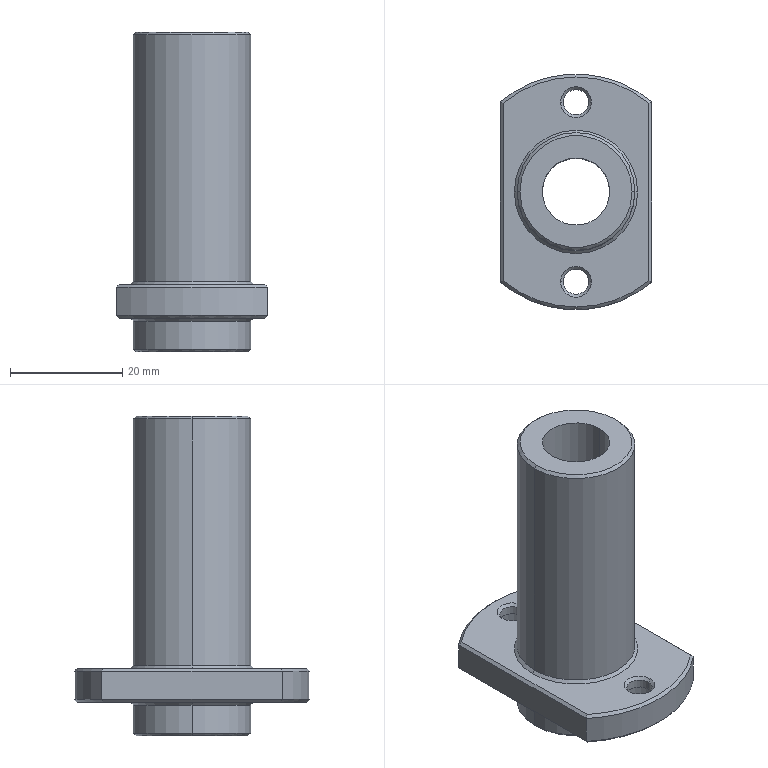Part | SolidWorks | features ICE 4, Chamfer 2, Extrusion 1, HoleWzd 1 | 1 solid | 48 faces | box 27 x 42 x 57 mm | volume 17013 mm3 | cone 20 | cylinder 16 | plane 12 | commonest cylinder face diameters 4.5 x4 8 x4 21 x4 12 x2 42 x2
STEP:
#1=CARTESIAN_POINT('',(4.,16.,6.5));
#2=VERTEX_POINT('',#1);
#3=CARTESIAN_POINT('',(-4.,16.,6.5));
#4=VERTEX_POINT('',#3);
#5=CARTESIAN_POINT('',(0.,16.,6.5));
#6=DIRECTION('',(0.,0.,-1.));
#7=DIRECTION('',(1.,0.,0.));
#8=AXIS2_PLACEMENT_3D('',#5,#6,#7);
#9=CIRCLE('',#8,4.);
#10=EDGE_CURVE('',#2,#4,#9,.T.);
#11=ORIENTED_EDGE('',*,*,#10,.F.);
#12=CARTESIAN_POINT('',(4.5,16.,6.));
#13=VERTEX_POINT('',#12);
#14=CARTESIAN_POINT('',(4.,16.,6.5));
#15=DIRECTION('',(0.7071,0.,-0.7071));
#16=VECTOR('',#15,1000.);
#17=LINE('',#14,#16);
#18=EDGE_CURVE('',#2,#13,#17,.T.);
#19=ORIENTED_EDGE('',*,*,#18,.T.);
#20=CARTESIAN_POINT('',(-4.5,16.,6.));
#21=VERTEX_POINT('',#20);
#22=CARTESIAN_POINT('',(0.,16.,6.));
#23=DIRECTION('',(0.,0.,1.));
#24=DIRECTION('',(1.,0.,0.));
#25=AXIS2_PLACEMENT_3D('',#22,#23,#24);
#26=CIRCLE('',#25,4.5);
#27=EDGE_CURVE('',#21,#13,#26,.T.);
#28=ORIENTED_EDGE('',*,*,#27,.F.);
#29=CARTESIAN_POINT('',(-4.,16.,6.5));
#30=DIRECTION('',(-0.7071,0.,-0.7071));
#31=VECTOR('',#30,1000.);
#32=LINE('',#29,#31);
#33=EDGE_CURVE('',#4,#21,#32,.T.);
#34=ORIENTED_EDGE('',*,*,#33,.F.);
#35=EDGE_LOOP('',(#11,#19,#28,#34));
#36=FACE_OUTER_BOUND('',#35,.T.);
#37=CARTESIAN_POINT('',(0.,16.,6.5));
#38=DIRECTION('',(0.,0.,-1.));
#39=DIRECTION('',(-1.,0.,0.));
#40=AXIS2_PLACEMENT_3D('',#37,#38,#39);
#41=CONICAL_SURFACE('',#40,4.,0.7854);
#42=ADVANCED_FACE('',(#36),#41,.F.);
#43=CARTESIAN_POINT('',(4.,-16.,6.5));
#44=VERTEX_POINT('',#43);
#45=CARTESIAN_POINT('',(-4.,-16.,6.5));
#46=VERTEX_POINT('',#45);
#47=CARTESIAN_POINT('',(0.,-16.,6.5));
#48=DIRECTION('',(0.,0.,-1.));
#49=DIRECTION('',(1.,0.,0.));
#50=AXIS2_PLACEMENT_3D('',#47,#48,#49);
#51=CIRCLE('',#50,4.);
#52=EDGE_CURVE('',#44,#46,#51,.T.);
#53=ORIENTED_EDGE('',*,*,#52,.F.);
#54=CARTESIAN_POINT('',(4.5,-16.,6.));
#55=VERTEX_POINT('',#54);
#56=CARTESIAN_POINT('',(4.,-16.,6.5));
#57=DIRECTION('',(0.7071,0.,-0.7071));
#58=VECTOR('',#57,1000.);
#59=LINE('',#56,#58);
#60=EDGE_CURVE('',#44,#55,#59,.T.);
#61=ORIENTED_EDGE('',*,*,#60,.T.);
#62=CARTESIAN_POINT('',(0.,-20.5,6.));
#63=VERTEX_POINT('',#62);
#64=CARTESIAN_POINT('',(0.,-16.,6.));
#65=DIRECTION('',(0.,0.,1.));
#66=DIRECTION('',(1.,0.,0.));
#67=AXIS2_PLACEMENT_3D('',#64,#65,#66);
#68=CIRCLE('',#67,4.5);
#69=EDGE_CURVE('',#63,#55,#68,.T.);
#70=ORIENTED_EDGE('',*,*,#69,.F.);
#71=CARTESIAN_POINT('',(-4.5,-16.,6.));
#72=VERTEX_POINT('',#71);
#73=CARTESIAN_POINT('',(0.,-16.,6.));
#74=DIRECTION('',(0.,0.,1.));
#75=DIRECTION('',(1.,0.,0.));
#76=AXIS2_PLACEMENT_3D('',#73,#74,#75);
#77=CIRCLE('',#76,4.5);
#78=EDGE_CURVE('',#72,#63,#77,.T.);
#79=ORIENTED_EDGE('',*,*,#78,.F.);
#80=CARTESIAN_POINT('',(-4.,-16.,6.5));
#81=DIRECTION('',(-0.7071,0.,-0.7071));
#82=VECTOR('',#81,1000.);
#83=LINE('',#80,#82);
#84=EDGE_CURVE('',#46,#72,#83,.T.);
#85=ORIENTED_EDGE('',*,*,#84,.F.);
#86=EDGE_LOOP('',(#53,#61,#70,#79,#85));
#87=FACE_OUTER_BOUND('',#86,.T.);
#88=CARTESIAN_POINT('',(0.,-16.,6.5));
#89=DIRECTION('',(0.,0.,-1.));
#90=DIRECTION('',(-1.,0.,0.));
#91=AXIS2_PLACEMENT_3D('',#88,#89,#90);
#92=CONICAL_SURFACE('',#91,4.,0.7854);
#93=ADVANCED_FACE('',(#87),#92,.F.);
#94=CARTESIAN_POINT('',(-10.5,0.,5.5));
#95=VERTEX_POINT('',#94);
#96=CARTESIAN_POINT('',(10.5,0.,5.5));
#97=VERTEX_POINT('',#96);
#98=CARTESIAN_POINT('',(0.,0.,5.5));
#99=DIRECTION('',(0.,0.,-1.));
#100=DIRECTION('',(1.,0.,0.));
#101=AXIS2_PLACEMENT_3D('',#98,#99,#100);
#102=CIRCLE('',#101,10.5);
#103=EDGE_CURVE('',#95,#97,#102,.T.);
#104=ORIENTED_EDGE('',*,*,#103,.F.);
#105=CARTESIAN_POINT('',(-11.,0.,6.));
#106=VERTEX_POINT('',#105);
#107=CARTESIAN_POINT('',(-11.,0.,6.));
#108=DIRECTION('',(-0.7071,0.,0.7071));
#109=VECTOR('',#108,1000.);
#110=LINE('',#107,#109);
#111=EDGE_CURVE('',#95,#106,#110,.T.);
#112=ORIENTED_EDGE('',*,*,#111,.T.);
#113=CARTESIAN_POINT('',(11.,0.,6.));
#114=VERTEX_POINT('',#113);
#115=CARTESIAN_POINT('',(0.,0.,6.));
#116=DIRECTION('',(0.,0.,1.));
#117=DIRECTION('',(1.,0.,0.));
#118=AXIS2_PLACEMENT_3D('',#115,#116,#117);
#119=CIRCLE('',#118,11.);
#120=EDGE_CURVE('',#114,#106,#119,.T.);
#121=ORIENTED_EDGE('',*,*,#120,.F.);
#122=CARTESIAN_POINT('',(11.,0.,6.));
#123=DIRECTION('',(0.7071,0.,0.7071));
#124=VECTOR('',#123,1000.);
#125=LINE('',#122,#124);
#126=EDGE_CURVE('',#97,#114,#125,.T.);
#127=ORIENTED_EDGE('',*,*,#126,.F.);
#128=EDGE_LOOP('',(#104,#112,#121,#127));
#129=FACE_OUTER_BOUND('',#128,.T.);
#130=CARTESIAN_POINT('',(0.,0.,6.));
#131=DIRECTION('',(0.,0.,1.));
#132=DIRECTION('',(1.,0.,0.));
#133=AXIS2_PLACEMENT_3D('',#130,#131,#132);
#134=CONICAL_SURFACE('',#133,11.,0.7854);
#135=ADVANCED_FACE('',(#129),#134,.T.);
#136=CARTESIAN_POINT('',(-2.25,16.,11.5));
#137=VERTEX_POINT('',#136);
#138=CARTESIAN_POINT('',(2.25,16.,11.5));
#139=VERTEX_POINT('',#138);
#140=CARTESIAN_POINT('',(0.,16.,11.5));
#141=DIRECTION('',(0.,0.,1.));
#142=DIRECTION('',(1.,0.,0.));
#143=AXIS2_PLACEMENT_3D('',#140,#141,#142);
#144=CIRCLE('',#143,2.25);
#145=EDGE_CURVE('',#137,#139,#144,.T.);
#146=ORIENTED_EDGE('',*,*,#145,.F.);
#147=CARTESIAN_POINT('',(-2.75,16.,12.));
#148=VERTEX_POINT('',#147);
#149=CARTESIAN_POINT('',(-2.25,16.,11.5));
#150=DIRECTION('',(-0.7071,0.,0.7071));
#151=VECTOR('',#150,1000.);
#152=LINE('',#149,#151);
#153=EDGE_CURVE('',#137,#148,#152,.T.);
#154=ORIENTED_EDGE('',*,*,#153,.T.);
#155=CARTESIAN_POINT('',(2.75,16.,12.));
#156=VERTEX_POINT('',#155);
#157=CARTESIAN_POINT('',(0.,16.,12.));
#158=DIRECTION('',(0.,0.,-1.));
#159=DIRECTION('',(1.,0.,0.));
#160=AXIS2_PLACEMENT_3D('',#157,#158,#159);
#161=CIRCLE('',#160,2.75);
#162=EDGE_CURVE('',#156,#148,#161,.T.);
#163=ORIENTED_EDGE('',*,*,#162,.F.);
#164=CARTESIAN_POINT('',(2.25,16.,11.5));
#165=DIRECTION('',(0.7071,0.,0.7071));
#166=VECTOR('',#165,1000.);
#167=LINE('',#164,#166);
#168=EDGE_CURVE('',#139,#156,#167,.T.);
#169=ORIENTED_EDGE('',*,*,#168,.F.);
#170=EDGE_LOOP('',(#146,#154,#163,#169));
#171=FACE_OUTER_BOUND('',#170,.T.);
#172=CARTESIAN_POINT('',(0.,16.,11.5));
#173=DIRECTION('',(0.,0.,1.));
#174=DIRECTION('',(1.,0.,0.));
#175=AXIS2_PLACEMENT_3D('',#172,#173,#174);
#176=CONICAL_SURFACE('',#175,2.25,0.7854);
#177=ADVANCED_FACE('',(#171),#176,.F.);
#178=CARTESIAN_POINT('',(-2.25,-16.,11.5));
#179=VERTEX_POINT('',#178);
#180=CARTESIAN_POINT('',(2.25,-16.,11.5));
#181=VERTEX_POINT('',#180);
#182=CARTESIAN_POINT('',(0.,-16.,11.5));
#183=DIRECTION('',(0.,0.,1.));
#184=DIRECTION('',(1.,0.,0.));
#185=AXIS2_PLACEMENT_3D('',#182,#183,#184);
#186=CIRCLE('',#185,2.25);
#187=EDGE_CURVE('',#179,#181,#186,.T.);
#188=ORIENTED_EDGE('',*,*,#187,.F.);
#189=CARTESIAN_POINT('',(-2.75,-16.,12.));
#190=VERTEX_POINT('',#189);
#191=CARTESIAN_POINT('',(-2.25,-16.,11.5));
#192=DIRECTION('',(-0.7071,0.,0.7071));
#193=VECTOR('',#192,1000.);
#194=LINE('',#191,#193);
#195=EDGE_CURVE('',#179,#190,#194,.T.);
#196=ORIENTED_EDGE('',*,*,#195,.T.);
#197=CARTESIAN_POINT('',(2.75,-16.,12.));
#198=VERTEX_POINT('',#197);
#199=CARTESIAN_POINT('',(0.,-16.,12.));
#200=DIRECTION('',(0.,0.,-1.));
#201=DIRECTION('',(1.,0.,0.));
#202=AXIS2_PLACEMENT_3D('',#199,#200,#201);
#203=CIRCLE('',#202,2.75);
#204=EDGE_CURVE('',#198,#190,#203,.T.);
#205=ORIENTED_EDGE('',*,*,#204,.F.);
#206=CARTESIAN_POINT('',(2.25,-16.,11.5));
#207=DIRECTION('',(0.7071,0.,0.7071));
#208=VECTOR('',#207,1000.);
#209=LINE('',#206,#208);
#210=EDGE_CURVE('',#181,#198,#209,.T.);
#211=ORIENTED_EDGE('',*,*,#210,.F.);
#212=EDGE_LOOP('',(#188,#196,#205,#211));
#213=FACE_OUTER_BOUND('',#212,.T.);
#214=CARTESIAN_POINT('',(0.,-16.,11.5));
#215=DIRECTION('',(0.,0.,1.));
#216=DIRECTION('',(1.,0.,0.));
#217=AXIS2_PLACEMENT_3D('',#214,#215,#216);
#218=CONICAL_SURFACE('',#217,2.25,0.7854);
#219=ADVANCED_FACE('',(#213),#218,.F.);
#220=CARTESIAN_POINT('',(10.5,0.,12.5));
#221=VERTEX_POINT('',#220);
#222=CARTESIAN_POINT('',(-10.5,0.,12.5));
#223=VERTEX_POINT('',#222);
#224=CARTESIAN_POINT('',(0.,0.,12.5));
#225=DIRECTION('',(0.,0.,1.));
#226=DIRECTION('',(1.,0.,0.));
#227=AXIS2_PLACEMENT_3D('',#224,#225,#226);
#228=CIRCLE('',#227,10.5);
#229=EDGE_CURVE('',#221,#223,#228,.T.);
#230=ORIENTED_EDGE('',*,*,#229,.F.);
#231=CARTESIAN_POINT('',(11.,0.,12.));
#232=VERTEX_POINT('',#231);
#233=CARTESIAN_POINT('',(10.5,0.,12.5));
#234=DIRECTION('',(0.7071,0.,-0.7071));
#235=VECTOR('',#234,1000.);
#236=LINE('',#233,#235);
#237=EDGE_CURVE('',#221,#232,#236,.T.);
#238=ORIENTED_EDGE('',*,*,#237,.T.);
#239=CARTESIAN_POINT('',(-11.,0.,12.));
#240=VERTEX_POINT('',#239);
#241=CARTESIAN_POINT('',(0.,0.,12.));
#242=DIRECTION('',(0.,0.,-1.));
#243=DIRECTION('',(1.,0.,0.));
#244=AXIS2_PLACEMENT_3D('',#241,#242,#243);
#245=CIRCLE('',#244,11.);
#246=EDGE_CURVE('',#240,#232,#245,.T.);
#247=ORIENTED_EDGE('',*,*,#246,.F.);
#248=CARTESIAN_POINT('',(-10.5,0.,12.5));
#249=DIRECTION('',(-0.7071,0.,-0.7071));
#250=VECTOR('',#249,1000.);
#251=LINE('',#248,#250);
#252=EDGE_CURVE('',#223,#240,#251,.T.);
#253=ORIENTED_EDGE('',*,*,#252,.F.);
#254=EDGE_LOOP('',(#230,#238,#247,#253));
#255=FACE_OUTER_BOUND('',#254,.T.);
#256=CARTESIAN_POINT('',(0.,0.,12.5));
#257=DIRECTION('',(0.,0.,-1.));
#258=DIRECTION('',(-1.,0.,0.));
#259=AXIS2_PLACEMENT_3D('',#256,#257,#258);
#260=CONICAL_SURFACE('',#259,10.5,0.7854);
#261=ADVANCED_FACE('',(#255),#260,.T.);
#262=CARTESIAN_POINT('',(10.,0.,57.));
#263=VERTEX_POINT('',#262);
#264=CARTESIAN_POINT('',(-10.,0.,57.));
#265=VERTEX_POINT('',#264);
#266=CARTESIAN_POINT('',(0.,0.,57.));
#267=DIRECTION('',(0.,0.,1.));
#268=DIRECTION('',(1.,0.,0.));
#269=AXIS2_PLACEMENT_3D('',#266,#267,#268);
#270=CIRCLE('',#269,10.);
#271=EDGE_CURVE('',#263,#265,#270,.T.);
#272=ORIENTED_EDGE('',*,*,#271,.F.);
#273=CARTESIAN_POINT('',(10.5,0.,56.5));
#274=VERTEX_POINT('',#273);
#275=CARTESIAN_POINT('',(10.,0.,57.));
#276=DIRECTION('',(0.7071,0.,-0.7071));
#277=VECTOR('',#276,1000.);
#278=LINE('',#275,#277);
#279=EDGE_CURVE('',#263,#274,#278,.T.);
#280=ORIENTED_EDGE('',*,*,#279,.T.);
#281=CARTESIAN_POINT('',(-10.5,0.,56.5));
#282=VERTEX_POINT('',#281);
#283=CARTESIAN_POINT('',(0.,0.,56.5));
#284=DIRECTION('',(0.,0.,-1.));
#285=DIRECTION('',(1.,0.,0.));
#286=AXIS2_PLACEMENT_3D('',#283,#284,#285);
#287=CIRCLE('',#286,10.5);
#288=EDGE_CURVE('',#282,#274,#287,.T.);
#289=ORIENTED_EDGE('',*,*,#288,.F.);
#290=CARTESIAN_POINT('',(-10.,0.,57.));
#291=DIRECTION('',(-0.7071,0.,-0.7071));
#292=VECTOR('',#291,1000.);
#293=LINE('',#290,#292);
#294=EDGE_CURVE('',#265,#282,#293,.T.);
#295=ORIENTED_EDGE('',*,*,#294,.F.);
#296=EDGE_LOOP('',(#272,#280,#289,#295));
#297=FACE_OUTER_BOUND('',#296,.T.);
#298=CARTESIAN_POINT('',(0.,0.,57.));
#299=DIRECTION('',(0.,0.,-1.));
#300=DIRECTION('',(-1.,0.,0.));
#301=AXIS2_PLACEMENT_3D('',#298,#299,#300);
#302=CONICAL_SURFACE('',#301,10.,0.7854);
#303=ADVANCED_FACE('',(#297),#302,.T.);
#304=CARTESIAN_POINT('',(-10.,0.,0.));
#305=VERTEX_POINT('',#304);
#306=CARTESIAN_POINT('',(10.,0.,0.));
#307=VERTEX_POINT('',#306);
#308=CARTESIAN_POINT('',(0.,0.,0.));
#309=DIRECTION('',(0.,0.,-1.));
#310=DIRECTION('',(1.,0.,0.));
#311=AXIS2_PLACEMENT_3D('',#308,#309,#310);
#312=CIRCLE('',#311,10.);
#313=EDGE_CURVE('',#305,#307,#312,.T.);
#314=ORIENTED_EDGE('',*,*,#313,.F.);
#315=CARTESIAN_POINT('',(-10.5,0.,0.5));
#316=VERTEX_POINT('',#315);
#317=CARTESIAN_POINT('',(-10.5,0.,0.5));
#318=DIRECTION('',(-0.7071,0.,0.7071));
#319=VECTOR('',#318,1000.);
#320=LINE('',#317,#319);
#321=EDGE_CURVE('',#305,#316,#320,.T.);
#322=ORIENTED_EDGE('',*,*,#321,.T.);
#323=CARTESIAN_POINT('',(10.5,0.,0.5));
#324=VERTEX_POINT('',#323);
#325=CARTESIAN_POINT('',(0.,0.,0.5));
#326=DIRECTION('',(0.,0.,1.));
#327=DIRECTION('',(1.,0.,0.));
#328=AXIS2_PLACEMENT_3D('',#325,#326,#327);
#329=CIRCLE('',#328,10.5);
#330=EDGE_CURVE('',#324,#316,#329,.T.);
#331=ORIENTED_EDGE('',*,*,#330,.F.);
#332=CARTESIAN_POINT('',(10.5,0.,0.5));
#333=DIRECTION('',(0.7071,0.,0.7071));
#334=VECTOR('',#333,1000.);
#335=LINE('',#332,#334);
#336=EDGE_CURVE('',#307,#324,#335,.T.);
#337=ORIENTED_EDGE('',*,*,#336,.F.);
#338=EDGE_LOOP('',(#314,#322,#331,#337));
#339=FACE_OUTER_BOUND('',#338,.T.);
#340=CARTESIAN_POINT('',(0.,0.,0.5));
#341=DIRECTION('',(0.,0.,1.));
#342=DIRECTION('',(1.,0.,0.));
#343=AXIS2_PLACEMENT_3D('',#340,#341,#342);
#344=CONICAL_SURFACE('',#343,10.5,0.7854);
#345=ADVANCED_FACE('',(#339),#344,.T.);
#346=CARTESIAN_POINT('',(4.,16.,10.));
#347=VERTEX_POINT('',#346);
#348=CARTESIAN_POINT('',(-4.,16.,10.));
#349=VERTEX_POINT('',#348);
#350=CARTESIAN_POINT('',(0.,16.,10.));
#351=DIRECTION('',(0.,0.,-1.));
#352=DIRECTION('',(-1.,0.,0.));
#353=AXIS2_PLACEMENT_3D('',#350,#351,#352);
#354=CIRCLE('',#353,4.);
#355=EDGE_CURVE('',#347,#349,#354,.T.);
#356=ORIENTED_EDGE('',*,*,#355,.F.);
#357=CARTESIAN_POINT('',(4.,16.,6.));
#358=DIRECTION('',(0.,0.,-1.));
#359=VECTOR('',#358,1000.);
#360=LINE('',#357,#359);
#361=EDGE_CURVE('',#347,#2,#360,.T.);
#362=ORIENTED_EDGE('',*,*,#361,.T.);
#363=ORIENTED_EDGE('',*,*,#10,.T.);
#364=CARTESIAN_POINT('',(-4.,16.,6.));
#365=DIRECTION('',(0.,0.,-1.));
#366=VECTOR('',#365,1000.);
#367=LINE('',#364,#366);
#368=EDGE_CURVE('',#349,#4,#367,.T.);
#369=ORIENTED_EDGE('',*,*,#368,.F.);
#370=EDGE_LOOP('',(#356,#362,#363,#369));
#371=FACE_OUTER_BOUND('',#370,.T.);
#372=CARTESIAN_POINT('',(0.,16.,6.));
#373=DIRECTION('',(0.,0.,-1.));
#374=DIRECTION('',(-1.,0.,0.));
#375=AXIS2_PLACEMENT_3D('',#372,#373,#374);
#376=CYLINDRICAL_SURFACE('',#375,4.);
#377=ADVANCED_FACE('',(#371),#376,.F.);
#378=ORIENTED_EDGE('',*,*,#145,.T.);
#379=CARTESIAN_POINT('',(2.25,16.,10.));
#380=VERTEX_POINT('',#379);
#381=CARTESIAN_POINT('',(2.25,16.,6.));
#382=DIRECTION('',(0.,0.,-1.));
#383=VECTOR('',#382,1000.);
#384=LINE('',#381,#383);
#385=EDGE_CURVE('',#139,#380,#384,.T.);
#386=ORIENTED_EDGE('',*,*,#385,.T.);
#387=CARTESIAN_POINT('',(-2.25,16.,10.));
#388=VERTEX_POINT('',#387);
#389=CARTESIAN_POINT('',(0.,16.,10.));
#390=DIRECTION('',(0.,0.,-1.));
#391=DIRECTION('',(-1.,0.,0.));
#392=AXIS2_PLACEMENT_3D('',#389,#390,#391);
#393=CIRCLE('',#392,2.25);
#394=EDGE_CURVE('',#380,#388,#393,.T.);
#395=ORIENTED_EDGE('',*,*,#394,.T.);
#396=CARTESIAN_POINT('',(-2.25,16.,6.));
#397=DIRECTION('',(0.,0.,-1.));
#398=VECTOR('',#397,1000.);
#399=LINE('',#396,#398);
#400=EDGE_CURVE('',#137,#388,#399,.T.);
#401=ORIENTED_EDGE('',*,*,#400,.F.);
#402=EDGE_LOOP('',(#378,#386,#395,#401));
#403=FACE_OUTER_BOUND('',#402,.T.);
#404=CARTESIAN_POINT('',(0.,16.,6.));
#405=DIRECTION('',(0.,0.,-1.));
#406=DIRECTION('',(-1.,0.,0.));
#407=AXIS2_PLACEMENT_3D('',#404,#405,#406);
#408=CYLINDRICAL_SURFACE('',#407,2.25);
#409=ADVANCED_FACE('',(#403),#408,.F.);
#410=CARTESIAN_POINT('',(4.,-16.,10.));
#411=VERTEX_POINT('',#410);
#412=CARTESIAN_POINT('',(-4.,-16.,10.));
#413=VERTEX_POINT('',#412);
#414=CARTESIAN_POINT('',(0.,-16.,10.));
#415=DIRECTION('',(0.,0.,-1.));
#416=DIRECTION('',(-1.,0.,0.));
#417=AXIS2_PLACEMENT_3D('',#414,#415,#416);
#418=CIRCLE('',#417,4.);
#419=EDGE_CURVE('',#411,#413,#418,.T.);
#420=ORIENTED_EDGE('',*,*,#419,.F.);
#421=CARTESIAN_POINT('',(4.,-16.,6.));
#422=DIRECTION('',(0.,0.,-1.));
#423=VECTOR('',#422,1000.);
#424=LINE('',#421,#423);
#425=EDGE_CURVE('',#411,#44,#424,.T.);
#426=ORIENTED_EDGE('',*,*,#425,.T.);
#427=ORIENTED_EDGE('',*,*,#52,.T.);
#428=CARTESIAN_POINT('',(-4.,-16.,6.));
#429=DIRECTION('',(0.,0.,-1.));
#430=VECTOR('',#429,1000.);
#431=LINE('',#428,#430);
#432=EDGE_CURVE('',#413,#46,#431,.T.);
#433=ORIENTED_EDGE('',*,*,#432,.F.);
#434=EDGE_LOOP('',(#420,#426,#427,#433));
#435=FACE_OUTER_BOUND('',#434,.T.);
#436=CARTESIAN_POINT('',(0.,-16.,6.));
#437=DIRECTION('',(0.,0.,-1.));
#438=DIRECTION('',(-1.,0.,0.));
#439=AXIS2_PLACEMENT_3D('',#436,#437,#438);
#440=CYLINDRICAL_SURFACE('',#439,4.);
#441=ADVANCED_FACE('',(#435),#440,.F.);
#442=ORIENTED_EDGE('',*,*,#187,.T.);
#443=CARTESIAN_POINT('',(2.25,-16.,10.));
#444=VERTEX_POINT('',#443);
#445=CARTESIAN_POINT('',(2.25,-16.,6.));
#446=DIRECTION('',(0.,0.,-1.));
#447=VECTOR('',#446,1000.);
#448=LINE('',#445,#447);
#449=EDGE_CURVE('',#181,#444,#448,.T.);
#450=ORIENTED_EDGE('',*,*,#449,.T.);
#451=CARTESIAN_POINT('',(-2.25,-16.,10.));
#452=VERTEX_POINT('',#451);
#453=CARTESIAN_POINT('',(0.,-16.,10.));
#454=DIRECTION('',(0.,0.,-1.));
#455=DIRECTION('',(-1.,0.,0.));
#456=AXIS2_PLACEMENT_3D('',#453,#454,#455);
#457=CIRCLE('',#456,2.25);
#458=EDGE_CURVE('',#444,#452,#457,.T.);
#459=ORIENTED_EDGE('',*,*,#458,.T.);
#460=CARTESIAN_POINT('',(-2.25,-16.,6.));
#461=DIRECTION('',(0.,0.,-1.));
#462=VECTOR('',#461,1000.);
#463=LINE('',#460,#462);
#464=EDGE_CURVE('',#179,#452,#463,.T.);
#465=ORIENTED_EDGE('',*,*,#464,.F.);
#466=EDGE_LOOP('',(#442,#450,#459,#465));
#467=FACE_OUTER_BOUND('',#466,.T.);
#468=CARTESIAN_POINT('',(0.,-16.,6.));
#469=DIRECTION('',(0.,0.,-1.));
#470=DIRECTION('',(-1.,0.,0.));
#471=AXIS2_PLACEMENT_3D('',#468,#469,#470);
#472=CYLINDRICAL_SURFACE('',#471,2.25);
#473=ADVANCED_FACE('',(#467),#472,.F.);
#474=CARTESIAN_POINT('',(-6.,0.,0.));
#475=VERTEX_POINT('',#474);
#476=CARTESIAN_POINT('',(6.,0.,0.));
#477=VERTEX_POINT('',#476);
#478=CARTESIAN_POINT('',(0.,0.,0.));
#479=DIRECTION('',(0.,0.,1.));
#480=DIRECTION('',(1.,0.,0.));
#481=AXIS2_PLACEMENT_3D('',#478,#479,#480);
#482=CIRCLE('',#481,6.);
#483=EDGE_CURVE('',#475,#477,#482,.T.);
#484=ORIENTED_EDGE('',*,*,#483,.F.);
#485=CARTESIAN_POINT('',(-6.,0.,57.));
#486=VERTEX_POINT('',#485);
#487=CARTESIAN_POINT('',(-6.,0.,0.));
#488=DIRECTION('',(0.,0.,1.));
#489=VECTOR('',#488,1000.);
#490=LINE('',#487,#489);
#491=EDGE_CURVE('',#475,#486,#490,.T.);
#492=ORIENTED_EDGE('',*,*,#491,.T.);
#493=CARTESIAN_POINT('',(6.,0.,57.));
#494=VERTEX_POINT('',#493);
#495=CARTESIAN_POINT('',(0.,0.,57.));
#496=DIRECTION('',(0.,0.,1.));
#497=DIRECTION('',(1.,0.,0.));
#498=AXIS2_PLACEMENT_3D('',#495,#496,#497);
#499=CIRCLE('',#498,6.);
#500=EDGE_CURVE('',#486,#494,#499,.T.);
#501=ORIENTED_EDGE('',*,*,#500,.T.);
#502=CARTESIAN_POINT('',(6.,0.,0.));
#503=DIRECTION('',(0.,0.,1.));
#504=VECTOR('',#503,1000.);
#505=LINE('',#502,#504);
#506=EDGE_CURVE('',#477,#494,#505,.T.);
#507=ORIENTED_EDGE('',*,*,#506,.F.);
#508=EDGE_LOOP('',(#484,#492,#501,#507));
#509=FACE_OUTER_BOUND('',#508,.T.);
#510=CARTESIAN_POINT('',(0.,0.,0.));
#511=DIRECTION('',(0.,0.,1.));
#512=DIRECTION('',(1.,0.,0.));
#513=AXIS2_PLACEMENT_3D('',#510,#511,#512);
#514=CYLINDRICAL_SURFACE('',#513,6.);
#515=ADVANCED_FACE('',(#509),#514,.F.);
#516=ORIENTED_EDGE('',*,*,#288,.T.);
#517=CARTESIAN_POINT('',(10.5,0.,57.));
#518=DIRECTION('',(0.,0.,-1.));
#519=VECTOR('',#518,1000.);
#520=LINE('',#517,#519);
#521=EDGE_CURVE('',#274,#221,#520,.T.);
#522=ORIENTED_EDGE('',*,*,#521,.T.);
#523=ORIENTED_EDGE('',*,*,#229,.T.);
#524=CARTESIAN_POINT('',(-10.5,0.,57.));
#525=DIRECTION('',(0.,0.,-1.));
#526=VECTOR('',#525,1000.);
#527=LINE('',#524,#526);
#528=EDGE_CURVE('',#282,#223,#527,.T.);
#529=ORIENTED_EDGE('',*,*,#528,.F.);
#530=EDGE_LOOP('',(#516,#522,#523,#529));
#531=FACE_OUTER_BOUND('',#530,.T.);
#532=CARTESIAN_POINT('',(0.,0.,57.));
#533=DIRECTION('',(0.,0.,-1.));
#534=DIRECTION('',(-1.,0.,0.));
#535=AXIS2_PLACEMENT_3D('',#532,#533,#534);
#536=CYLINDRICAL_SURFACE('',#535,10.5);
#537=ADVANCED_FACE('',(#531),#536,.T.);
#538=ORIENTED_EDGE('',*,*,#103,.T.);
#539=CARTESIAN_POINT('',(10.5,0.,6.));
#540=DIRECTION('',(0.,0.,-1.));
#541=VECTOR('',#540,1000.);
#542=LINE('',#539,#541);
#543=EDGE_CURVE('',#97,#324,#542,.T.);
#544=ORIENTED_EDGE('',*,*,#543,.T.);
#545=ORIENTED_EDGE('',*,*,#330,.T.);
#546=CARTESIAN_POINT('',(-10.5,0.,6.));
#547=DIRECTION('',(0.,0.,-1.));
#548=VECTOR('',#547,1000.);
#549=LINE('',#546,#548);
#550=EDGE_CURVE('',#95,#316,#549,.T.);
#551=ORIENTED_EDGE('',*,*,#550,.F.);
#552=EDGE_LOOP('',(#538,#544,#545,#551));
#553=FACE_OUTER_BOUND('',#552,.T.);
#554=CARTESIAN_POINT('',(0.,0.,6.));
#555=DIRECTION('',(0.,0.,-1.));
#556=DIRECTION('',(-1.,0.,0.));
#557=AXIS2_PLACEMENT_3D('',#554,#555,#556);
#558=CYLINDRICAL_SURFACE('',#557,10.5);
#559=ADVANCED_FACE('',(#553),#558,.T.);
#560=CARTESIAN_POINT('',(13.,15.851,12.));
#561=VERTEX_POINT('',#560);
#562=CARTESIAN_POINT('',(-13.,15.851,12.));
#563=VERTEX_POINT('',#562);
#564=CARTESIAN_POINT('',(0.,0.,12.));
#565=DIRECTION('',(0.,0.,1.));
#566=DIRECTION('',(1.,0.,0.));
#567=AXIS2_PLACEMENT_3D('',#564,#565,#566);
#568=CIRCLE('',#567,20.5);
#569=EDGE_CURVE('',#561,#563,#568,.T.);
#570=ORIENTED_EDGE('',*,*,#569,.T.);
#571=CARTESIAN_POINT('',(-13.,-15.851,12.));
#572=VERTEX_POINT('',#571);
#573=CARTESIAN_POINT('',(-13.,0.,12.));
#574=DIRECTION('',(0.,-1.,0.));
#575=VECTOR('',#574,1000.);
#576=LINE('',#573,#575);
#577=EDGE_CURVE('',#563,#572,#576,.T.);
#578=ORIENTED_EDGE('',*,*,#577,.T.);
#579=CARTESIAN_POINT('',(13.,-15.851,12.));
#580=VERTEX_POINT('',#579);
#581=CARTESIAN_POINT('',(0.,0.,12.));
#582=DIRECTION('',(0.,0.,1.));
#583=DIRECTION('',(1.,0.,0.));
#584=AXIS2_PLACEMENT_3D('',#581,#582,#583);
#585=CIRCLE('',#584,20.5);
#586=EDGE_CURVE('',#572,#580,#585,.T.);
#587=ORIENTED_EDGE('',*,*,#586,.T.);
#588=CARTESIAN_POINT('',(13.,0.,12.));
#589=DIRECTION('',(0.,1.,0.));
#590=VECTOR('',#589,1000.);
#591=LINE('',#588,#590);
#592=EDGE_CURVE('',#580,#561,#591,.T.);
#593=ORIENTED_EDGE('',*,*,#592,.T.);
#594=EDGE_LOOP('',(#570,#578,#587,#593));
#595=FACE_OUTER_BOUND('',#594,.T.);
#596=ORIENTED_EDGE('',*,*,#246,.T.);
#597=CARTESIAN_POINT('',(0.,0.,12.));
#598=DIRECTION('',(0.,0.,-1.));
#599=DIRECTION('',(1.,0.,0.));
#600=AXIS2_PLACEMENT_3D('',#597,#598,#599);
#601=CIRCLE('',#600,11.);
#602=EDGE_CURVE('',#232,#240,#601,.T.);
#603=ORIENTED_EDGE('',*,*,#602,.T.);
#604=EDGE_LOOP('',(#596,#603));
#605=FACE_BOUND('',#604,.T.);
#606=ORIENTED_EDGE('',*,*,#204,.T.);
#607=CARTESIAN_POINT('',(0.,-16.,12.));
#608=DIRECTION('',(0.,0.,-1.));
#609=DIRECTION('',(1.,0.,0.));
#610=AXIS2_PLACEMENT_3D('',#607,#608,#609);
#611=CIRCLE('',#610,2.75);
#612=EDGE_CURVE('',#190,#198,#611,.T.);
#613=ORIENTED_EDGE('',*,*,#612,.T.);
#614=EDGE_LOOP('',(#606,#613));
#615=FACE_BOUND('',#614,.T.);
#616=ORIENTED_EDGE('',*,*,#162,.T.);
#617=CARTESIAN_POINT('',(0.,16.,12.));
#618=DIRECTION('',(0.,0.,-1.));
#619=DIRECTION('',(1.,0.,0.));
#620=AXIS2_PLACEMENT_3D('',#617,#618,#619);
#621=CIRCLE('',#620,2.75);
#622=EDGE_CURVE('',#148,#156,#621,.T.);
#623=ORIENTED_EDGE('',*,*,#622,.T.);
#624=EDGE_LOOP('',(#616,#623));
#625=FACE_BOUND('',#624,.T.);
#626=CARTESIAN_POINT('',(0.,0.,12.));
#627=DIRECTION('',(0.,0.,1.));
#628=DIRECTION('',(1.,0.,0.));
#629=AXIS2_PLACEMENT_3D('',#626,#627,#628);
#630=PLANE('',#629);
#631=ADVANCED_FACE('',(#595,#605,#615,#625),#630,.T.);
#632=ORIENTED_EDGE('',*,*,#120,.T.);
#633=CARTESIAN_POINT('',(0.,0.,6.));
#634=DIRECTION('',(0.,0.,1.));
#635=DIRECTION('',(1.,0.,0.));
#636=AXIS2_PLACEMENT_3D('',#633,#634,#635);
#637=CIRCLE('',#636,11.);
#638=EDGE_CURVE('',#106,#114,#637,.T.);
#639=ORIENTED_EDGE('',*,*,#638,.T.);
#640=EDGE_LOOP('',(#632,#639));
#641=FACE_BOUND('',#640,.T.);
#642=CARTESIAN_POINT('',(-13.,-15.851,6.));
#643=VERTEX_POINT('',#642);
#644=CARTESIAN_POINT('',(-13.,15.851,6.));
#645=VERTEX_POINT('',#644);
#646=CARTESIAN_POINT('',(-13.,16.086,6.));
#647=DIRECTION('',(0.,1.,0.));
#648=VECTOR('',#647,1000.);
#649=LINE('',#646,#648);
#650=EDGE_CURVE('',#643,#645,#649,.T.);
#651=ORIENTED_EDGE('',*,*,#650,.T.);
#652=CARTESIAN_POINT('',(0.,20.5,6.));
#653=VERTEX_POINT('',#652);
#654=CARTESIAN_POINT('',(0.,0.,6.));
#655=DIRECTION('',(0.,0.,-1.));
#656=DIRECTION('',(1.,0.,0.));
#657=AXIS2_PLACEMENT_3D('',#654,#655,#656);
#658=CIRCLE('',#657,20.5);
#659=EDGE_CURVE('',#645,#653,#658,.T.);
#660=ORIENTED_EDGE('',*,*,#659,.T.);
#661=CARTESIAN_POINT('',(0.,16.,6.));
#662=DIRECTION('',(0.,0.,1.));
#663=DIRECTION('',(1.,0.,0.));
#664=AXIS2_PLACEMENT_3D('',#661,#662,#663);
#665=CIRCLE('',#664,4.5);
#666=EDGE_CURVE('',#653,#21,#665,.T.);
#667=ORIENTED_EDGE('',*,*,#666,.T.);
#668=ORIENTED_EDGE('',*,*,#27,.T.);
#669=CARTESIAN_POINT('',(0.,16.,6.));
#670=DIRECTION('',(0.,0.,1.));
#671=DIRECTION('',(1.,0.,0.));
#672=AXIS2_PLACEMENT_3D('',#669,#670,#671);
#673=CIRCLE('',#672,4.5);
#674=EDGE_CURVE('',#13,#653,#673,.T.);
#675=ORIENTED_EDGE('',*,*,#674,.T.);
#676=CARTESIAN_POINT('',(13.,15.851,6.));
#677=VERTEX_POINT('',#676);
#678=CARTESIAN_POINT('',(0.,0.,6.));
#679=DIRECTION('',(0.,0.,-1.));
#680=DIRECTION('',(1.,0.,0.));
#681=AXIS2_PLACEMENT_3D('',#678,#679,#680);
#682=CIRCLE('',#681,20.5);
#683=EDGE_CURVE('',#653,#677,#682,.T.);
#684=ORIENTED_EDGE('',*,*,#683,.T.);
#685=CARTESIAN_POINT('',(13.,-15.851,6.));
#686=VERTEX_POINT('',#685);
#687=CARTESIAN_POINT('',(13.,-16.086,6.));
#688=DIRECTION('',(0.,-1.,0.));
#689=VECTOR('',#688,1000.);
#690=LINE('',#687,#689);
#691=EDGE_CURVE('',#677,#686,#690,.T.);
#692=ORIENTED_EDGE('',*,*,#691,.T.);
#693=CARTESIAN_POINT('',(0.,0.,6.));
#694=DIRECTION('',(0.,0.,-1.));
#695=DIRECTION('',(1.,0.,0.));
#696=AXIS2_PLACEMENT_3D('',#693,#694,#695);
#697=CIRCLE('',#696,20.5);
#698=EDGE_CURVE('',#686,#63,#697,.T.);
#699=ORIENTED_EDGE('',*,*,#698,.T.);
#700=ORIENTED_EDGE('',*,*,#69,.T.);
#701=CARTESIAN_POINT('',(0.,-16.,6.));
#702=DIRECTION('',(0.,0.,1.));
#703=DIRECTION('',(1.,0.,0.));
#704=AXIS2_PLACEMENT_3D('',#701,#702,#703);
#705=CIRCLE('',#704,4.5);
#706=EDGE_CURVE('',#55,#72,#705,.T.);
#707=ORIENTED_EDGE('',*,*,#706,.T.);
#708=ORIENTED_EDGE('',*,*,#78,.T.);
#709=CARTESIAN_POINT('',(0.,0.,6.));
#710=DIRECTION('',(0.,0.,-1.));
#711=DIRECTION('',(1.,0.,0.));
#712=AXIS2_PLACEMENT_3D('',#709,#710,#711);
#713=CIRCLE('',#712,20.5);
#714=EDGE_CURVE('',#63,#643,#713,.T.);
#715=ORIENTED_EDGE('',*,*,#714,.T.);
#716=EDGE_LOOP('',(#651,#660,#667,#668,#675,#684,#692,#699,#700,#707,#708,#715));
#717=FACE_OUTER_BOUND('',#716,.T.);
#718=CARTESIAN_POINT('',(0.,0.,6.));
#719=DIRECTION('',(0.,0.,1.));
#720=DIRECTION('',(1.,0.,0.));
#721=AXIS2_PLACEMENT_3D('',#718,#719,#720);
#722=PLANE('',#721);
#723=ADVANCED_FACE('',(#641,#717),#722,.F.);
#724=CARTESIAN_POINT('',(13.5,-16.086,11.5));
#725=VERTEX_POINT('',#724);
#726=CARTESIAN_POINT('',(13.5,-16.086,6.5));
#727=VERTEX_POINT('',#726);
#728=CARTESIAN_POINT('',(13.5,-16.086,12.));
#729=DIRECTION('',(0.,0.,-1.));
#730=VECTOR('',#729,1000.);
#731=LINE('',#728,#730);
#732=EDGE_CURVE('',#725,#727,#731,.T.);
#733=ORIENTED_EDGE('',*,*,#732,.F.);
#734=CARTESIAN_POINT('',(-13.5,-16.086,11.5));
#735=VERTEX_POINT('',#734);
#736=CARTESIAN_POINT('',(0.,0.,11.5));
#737=DIRECTION('',(0.,0.,-1.));
#738=DIRECTION('',(1.,0.,0.));
#739=AXIS2_PLACEMENT_3D('',#736,#737,#738);
#740=CIRCLE('',#739,21.);
#741=EDGE_CURVE('',#725,#735,#740,.T.);
#742=ORIENTED_EDGE('',*,*,#741,.T.);
#743=CARTESIAN_POINT('',(-13.5,-16.086,6.5));
#744=VERTEX_POINT('',#743);
#745=CARTESIAN_POINT('',(-13.5,-16.086,12.));
#746=DIRECTION('',(0.,0.,1.));
#747=VECTOR('',#746,1000.);
#748=LINE('',#745,#747);
#749=EDGE_CURVE('',#744,#735,#748,.T.);
#750=ORIENTED_EDGE('',*,*,#749,.F.);
#751=CARTESIAN_POINT('',(0.,0.,6.5));
#752=DIRECTION('',(0.,0.,1.));
#753=DIRECTION('',(1.,0.,0.));
#754=AXIS2_PLACEMENT_3D('',#751,#752,#753);
#755=CIRCLE('',#754,21.);
#756=EDGE_CURVE('',#744,#727,#755,.T.);
#757=ORIENTED_EDGE('',*,*,#756,.T.);
#758=EDGE_LOOP('',(#733,#742,#750,#757));
#759=FACE_OUTER_BOUND('',#758,.T.);
#760=CARTESIAN_POINT('',(0.,0.,12.));
#761=DIRECTION('',(0.,0.,-1.));
#762=DIRECTION('',(-1.,0.,0.));
#763=AXIS2_PLACEMENT_3D('',#760,#761,#762);
#764=CYLINDRICAL_SURFACE('',#763,21.);
#765=ADVANCED_FACE('',(#759),#764,.T.);
#766=CARTESIAN_POINT('',(-13.5,16.086,11.5));
#767=VERTEX_POINT('',#766);
#768=CARTESIAN_POINT('',(-13.5,16.086,6.5));
#769=VERTEX_POINT('',#768);
#770=CARTESIAN_POINT('',(-13.5,16.086,12.));
#771=DIRECTION('',(0.,0.,-1.));
#772=VECTOR('',#771,1000.);
#773=LINE('',#770,#772);
#774=EDGE_CURVE('',#767,#769,#773,.T.);
#775=ORIENTED_EDGE('',*,*,#774,.F.);
#776=CARTESIAN_POINT('',(13.5,16.086,11.5));
#777=VERTEX_POINT('',#776);
#778=CARTESIAN_POINT('',(0.,0.,11.5));
#779=DIRECTION('',(0.,0.,-1.));
#780=DIRECTION('',(1.,0.,0.));
#781=AXIS2_PLACEMENT_3D('',#778,#779,#780);
#782=CIRCLE('',#781,21.);
#783=EDGE_CURVE('',#767,#777,#782,.T.);
#784=ORIENTED_EDGE('',*,*,#783,.T.);
#785=CARTESIAN_POINT('',(13.5,16.086,6.5));
#786=VERTEX_POINT('',#785);
#787=CARTESIAN_POINT('',(13.5,16.086,12.));
#788=DIRECTION('',(0.,0.,1.));
#789=VECTOR('',#788,1000.);
#790=LINE('',#787,#789);
#791=EDGE_CURVE('',#786,#777,#790,.T.);
#792=ORIENTED_EDGE('',*,*,#791,.F.);
#793=CARTESIAN_POINT('',(0.,0.,6.5));
#794=DIRECTION('',(0.,0.,1.));
#795=DIRECTION('',(1.,0.,0.));
#796=AXIS2_PLACEMENT_3D('',#793,#794,#795);
#797=CIRCLE('',#796,21.);
#798=EDGE_CURVE('',#786,#769,#797,.T.);
#799=ORIENTED_EDGE('',*,*,#798,.T.);
#800=EDGE_LOOP('',(#775,#784,#792,#799));
#801=FACE_OUTER_BOUND('',#800,.T.);
#802=CARTESIAN_POINT('',(0.,0.,12.));
#803=DIRECTION('',(0.,0.,-1.));
#804=DIRECTION('',(-1.,0.,0.));
#805=AXIS2_PLACEMENT_3D('',#802,#803,#804);
#806=CYLINDRICAL_SURFACE('',#805,21.);
#807=ADVANCED_FACE('',(#801),#806,.T.);
#808=ORIENTED_EDGE('',*,*,#543,.F.);
#809=CARTESIAN_POINT('',(0.,0.,5.5));
#810=DIRECTION('',(0.,0.,-1.));
#811=DIRECTION('',(1.,0.,0.));
#812=AXIS2_PLACEMENT_3D('',#809,#810,#811);
#813=CIRCLE('',#812,10.5);
#814=EDGE_CURVE('',#97,#95,#813,.T.);
#815=ORIENTED_EDGE('',*,*,#814,.T.);
#816=ORIENTED_EDGE('',*,*,#550,.T.);
#817=CARTESIAN_POINT('',(0.,0.,0.5));
#818=DIRECTION('',(0.,0.,1.));
#819=DIRECTION('',(1.,0.,0.));
#820=AXIS2_PLACEMENT_3D('',#817,#818,#819);
#821=CIRCLE('',#820,10.5);
#822=EDGE_CURVE('',#316,#324,#821,.T.);
#823=ORIENTED_EDGE('',*,*,#822,.T.);
#824=EDGE_LOOP('',(#808,#815,#816,#823));
#825=FACE_OUTER_BOUND('',#824,.T.);
#826=CARTESIAN_POINT('',(0.,0.,6.));
#827=DIRECTION('',(0.,0.,-1.));
#828=DIRECTION('',(-1.,0.,0.));
#829=AXIS2_PLACEMENT_3D('',#826,#827,#828);
#830=CYLINDRICAL_SURFACE('',#829,10.5);
#831=ADVANCED_FACE('',(#825),#830,.T.);
#832=CARTESIAN_POINT('',(0.,0.,0.));
#833=DIRECTION('',(0.,0.,-1.));
#834=DIRECTION('',(1.,0.,0.));
#835=AXIS2_PLACEMENT_3D('',#832,#833,#834);
#836=CIRCLE('',#835,10.);
#837=EDGE_CURVE('',#307,#305,#836,.T.);
#838=ORIENTED_EDGE('',*,*,#837,.T.);
#839=ORIENTED_EDGE('',*,*,#313,.T.);
#840=EDGE_LOOP('',(#838,#839));
#841=FACE_OUTER_BOUND('',#840,.T.);
#842=CARTESIAN_POINT('',(0.,0.,0.));
#843=DIRECTION('',(0.,0.,1.));
#844=DIRECTION('',(1.,0.,0.));
#845=AXIS2_PLACEMENT_3D('',#842,#843,#844);
#846=CIRCLE('',#845,6.);
#847=EDGE_CURVE('',#477,#475,#846,.T.);
#848=ORIENTED_EDGE('',*,*,#847,.T.);
#849=ORIENTED_EDGE('',*,*,#483,.T.);
#850=EDGE_LOOP('',(#848,#849));
#851=FACE_BOUND('',#850,.T.);
#852=CARTESIAN_POINT('',(0.,0.,0.));
#853=DIRECTION('',(0.,0.,1.));
#854=DIRECTION('',(1.,0.,0.));
#855=AXIS2_PLACEMENT_3D('',#852,#853,#854);
#856=PLANE('',#855);
#857=ADVANCED_FACE('',(#841,#851),#856,.F.);
#858=ORIENTED_EDGE('',*,*,#521,.F.);
#859=CARTESIAN_POINT('',(0.,0.,56.5));
#860=DIRECTION('',(0.,0.,-1.));
#861=DIRECTION('',(1.,0.,0.));
#862=AXIS2_PLACEMENT_3D('',#859,#860,#861);
#863=CIRCLE('',#862,10.5);
#864=EDGE_CURVE('',#274,#282,#863,.T.);
#865=ORIENTED_EDGE('',*,*,#864,.T.);
#866=ORIENTED_EDGE('',*,*,#528,.T.);
#867=CARTESIAN_POINT('',(0.,0.,12.5));
#868=DIRECTION('',(0.,0.,1.));
#869=DIRECTION('',(1.,0.,0.));
#870=AXIS2_PLACEMENT_3D('',#867,#868,#869);
#871=CIRCLE('',#870,10.5);
#872=EDGE_CURVE('',#223,#221,#871,.T.);
#873=ORIENTED_EDGE('',*,*,#872,.T.);
#874=EDGE_LOOP('',(#858,#865,#866,#873));
#875=FACE_OUTER_BOUND('',#874,.T.);
#876=CARTESIAN_POINT('',(0.,0.,57.));
#877=DIRECTION('',(0.,0.,-1.));
#878=DIRECTION('',(-1.,0.,0.));
#879=AXIS2_PLACEMENT_3D('',#876,#877,#878);
#880=CYLINDRICAL_SURFACE('',#879,10.5);
#881=ADVANCED_FACE('',(#875),#880,.T.);
#882=CARTESIAN_POINT('',(0.,0.,57.));
#883=DIRECTION('',(0.,0.,1.));
#884=DIRECTION('',(1.,0.,0.));
#885=AXIS2_PLACEMENT_3D('',#882,#883,#884);
#886=CIRCLE('',#885,10.);
#887=EDGE_CURVE('',#265,#263,#886,.T.);
#888=ORIENTED_EDGE('',*,*,#887,.T.);
#889=ORIENTED_EDGE('',*,*,#271,.T.);
#890=EDGE_LOOP('',(#888,#889));
#891=FACE_OUTER_BOUND('',#890,.T.);
#892=CARTESIAN_POINT('',(0.,0.,57.));
#893=DIRECTION('',(0.,0.,1.));
#894=DIRECTION('',(1.,0.,0.));
#895=AXIS2_PLACEMENT_3D('',#892,#893,#894);
#896=CIRCLE('',#895,6.);
#897=EDGE_CURVE('',#494,#486,#896,.T.);
#898=ORIENTED_EDGE('',*,*,#897,.F.);
#899=ORIENTED_EDGE('',*,*,#500,.F.);
#900=EDGE_LOOP('',(#898,#899));
#901=FACE_BOUND('',#900,.T.);
#902=CARTESIAN_POINT('',(0.,0.,57.));
#903=DIRECTION('',(0.,0.,1.));
#904=DIRECTION('',(1.,0.,0.));
#905=AXIS2_PLACEMENT_3D('',#902,#903,#904);
#906=PLANE('',#905);
#907=ADVANCED_FACE('',(#891,#901),#906,.T.);
#908=ORIENTED_EDGE('',*,*,#491,.F.);
#909=ORIENTED_EDGE('',*,*,#847,.F.);
#910=ORIENTED_EDGE('',*,*,#506,.T.);
#911=ORIENTED_EDGE('',*,*,#897,.T.);
#912=EDGE_LOOP('',(#908,#909,#910,#911));
#913=FACE_OUTER_BOUND('',#912,.T.);
#914=CARTESIAN_POINT('',(0.,0.,0.));
#915=DIRECTION('',(0.,0.,1.));
#916=DIRECTION('',(1.,0.,0.));
#917=AXIS2_PLACEMENT_3D('',#914,#915,#916);
#918=CYLINDRICAL_SURFACE('',#917,6.);
#919=ADVANCED_FACE('',(#913),#918,.F.);
#920=ORIENTED_EDGE('',*,*,#749,.T.);
#921=CARTESIAN_POINT('',(-13.5,25.,11.5));
#922=DIRECTION('',(0.,1.,0.));
#923=VECTOR('',#922,1000.);
#924=LINE('',#921,#923);
#925=EDGE_CURVE('',#735,#767,#924,.T.);
#926=ORIENTED_EDGE('',*,*,#925,.T.);
#927=ORIENTED_EDGE('',*,*,#774,.T.);
#928=CARTESIAN_POINT('',(-13.5,-16.086,6.5));
#929=DIRECTION('',(0.,-1.,0.));
#930=VECTOR('',#929,1000.);
#931=LINE('',#928,#930);
#932=EDGE_CURVE('',#769,#744,#931,.T.);
#933=ORIENTED_EDGE('',*,*,#932,.T.);
#934=EDGE_LOOP('',(#920,#926,#927,#933));
#935=FACE_OUTER_BOUND('',#934,.T.);
#936=CARTESIAN_POINT('',(-13.5,25.,-33.));
#937=DIRECTION('',(-1.,0.,0.));
#938=DIRECTION('',(0.,-1.,0.));
#939=AXIS2_PLACEMENT_3D('',#936,#937,#938);
#940=PLANE('',#939);
#941=ADVANCED_FACE('',(#935),#940,.T.);
#942=ORIENTED_EDGE('',*,*,#791,.T.);
#943=CARTESIAN_POINT('',(13.5,25.,11.5));
#944=DIRECTION('',(0.,-1.,0.));
#945=VECTOR('',#944,1000.);
#946=LINE('',#943,#945);
#947=EDGE_CURVE('',#777,#725,#946,.T.);
#948=ORIENTED_EDGE('',*,*,#947,.T.);
#949=ORIENTED_EDGE('',*,*,#732,.T.);
#950=CARTESIAN_POINT('',(13.5,16.086,6.5));
#951=DIRECTION('',(0.,1.,0.));
#952=VECTOR('',#951,1000.);
#953=LINE('',#950,#952);
#954=EDGE_CURVE('',#727,#786,#953,.T.);
#955=ORIENTED_EDGE('',*,*,#954,.T.);
#956=EDGE_LOOP('',(#942,#948,#949,#955));
#957=FACE_OUTER_BOUND('',#956,.T.);
#958=CARTESIAN_POINT('',(13.5,25.,-33.));
#959=DIRECTION('',(1.,0.,0.));
#960=DIRECTION('',(0.,1.,0.));
#961=AXIS2_PLACEMENT_3D('',#958,#959,#960);
#962=PLANE('',#961);
#963=ADVANCED_FACE('',(#957),#962,.T.);
#964=ORIENTED_EDGE('',*,*,#449,.F.);
#965=CARTESIAN_POINT('',(0.,-16.,11.5));
#966=DIRECTION('',(0.,0.,1.));
#967=DIRECTION('',(1.,0.,0.));
#968=AXIS2_PLACEMENT_3D('',#965,#966,#967);
#969=CIRCLE('',#968,2.25);
#970=EDGE_CURVE('',#181,#179,#969,.T.);
#971=ORIENTED_EDGE('',*,*,#970,.T.);
#972=ORIENTED_EDGE('',*,*,#464,.T.);
#973=CARTESIAN_POINT('',(0.,-16.,10.));
#974=DIRECTION('',(0.,0.,-1.));
#975=DIRECTION('',(-1.,0.,0.));
#976=AXIS2_PLACEMENT_3D('',#973,#974,#975);
#977=CIRCLE('',#976,2.25);
#978=EDGE_CURVE('',#452,#444,#977,.T.);
#979=ORIENTED_EDGE('',*,*,#978,.T.);
#980=EDGE_LOOP('',(#964,#971,#972,#979));
#981=FACE_OUTER_BOUND('',#980,.T.);
#982=CARTESIAN_POINT('',(0.,-16.,6.));
#983=DIRECTION('',(0.,0.,-1.));
#984=DIRECTION('',(-1.,0.,0.));
#985=AXIS2_PLACEMENT_3D('',#982,#983,#984);
#986=CYLINDRICAL_SURFACE('',#985,2.25);
#987=ADVANCED_FACE('',(#981),#986,.F.);
#988=ORIENTED_EDGE('',*,*,#978,.F.);
#989=ORIENTED_EDGE('',*,*,#458,.F.);
#990=EDGE_LOOP('',(#988,#989));
#991=FACE_BOUND('',#990,.T.);
#992=CARTESIAN_POINT('',(0.,-16.,10.));
#993=DIRECTION('',(0.,0.,-1.));
#994=DIRECTION('',(-1.,0.,0.));
#995=AXIS2_PLACEMENT_3D('',#992,#993,#994);
#996=CIRCLE('',#995,4.);
#997=EDGE_CURVE('',#413,#411,#996,.T.);
#998=ORIENTED_EDGE('',*,*,#997,.T.);
#999=ORIENTED_EDGE('',*,*,#419,.T.);
#1000=EDGE_LOOP('',(#998,#999));
#1001=FACE_OUTER_BOUND('',#1000,.T.);
#1002=CARTESIAN_POINT('',(2.25,-16.,10.));
#1003=DIRECTION('',(0.,0.,1.));
#1004=DIRECTION('',(1.,0.,0.));
#1005=AXIS2_PLACEMENT_3D('',#1002,#1003,#1004);
#1006=PLANE('',#1005);
#1007=ADVANCED_FACE('',(#991,#1001),#1006,.F.);
#1008=ORIENTED_EDGE('',*,*,#425,.F.);
#1009=ORIENTED_EDGE('',*,*,#997,.F.);
#1010=ORIENTED_EDGE('',*,*,#432,.T.);
#1011=CARTESIAN_POINT('',(0.,-16.,6.5));
#1012=DIRECTION('',(0.,0.,-1.));
#1013=DIRECTION('',(1.,0.,0.));
#1014=AXIS2_PLACEMENT_3D('',#1011,#1012,#1013);
#1015=CIRCLE('',#1014,4.);
#1016=EDGE_CURVE('',#46,#44,#1015,.T.);
#1017=ORIENTED_EDGE('',*,*,#1016,.T.);
#1018=EDGE_LOOP('',(#1008,#1009,#1010,#1017));
#1019=FACE_OUTER_BOUND('',#1018,.T.);
#1020=CARTESIAN_POINT('',(0.,-16.,6.));
#1021=DIRECTION('',(0.,0.,-1.));
#1022=DIRECTION('',(-1.,0.,0.));
#1023=AXIS2_PLACEMENT_3D('',#1020,#1021,#1022);
#1024=CYLINDRICAL_SURFACE('',#1023,4.);
#1025=ADVANCED_FACE('',(#1019),#1024,.F.);
#1026=ORIENTED_EDGE('',*,*,#385,.F.);
#1027=CARTESIAN_POINT('',(0.,16.,11.5));
#1028=DIRECTION('',(0.,0.,1.));
#1029=DIRECTION('',(1.,0.,0.));
#1030=AXIS2_PLACEMENT_3D('',#1027,#1028,#1029);
#1031=CIRCLE('',#1030,2.25);
#1032=EDGE_CURVE('',#139,#137,#1031,.T.);
#1033=ORIENTED_EDGE('',*,*,#1032,.T.);
#1034=ORIENTED_EDGE('',*,*,#400,.T.);
#1035=CARTESIAN_POINT('',(0.,16.,10.));
#1036=DIRECTION('',(0.,0.,-1.));
#1037=DIRECTION('',(-1.,0.,0.));
#1038=AXIS2_PLACEMENT_3D('',#1035,#1036,#1037);
#1039=CIRCLE('',#1038,2.25);
#1040=EDGE_CURVE('',#388,#380,#1039,.T.);
#1041=ORIENTED_EDGE('',*,*,#1040,.T.);
#1042=EDGE_LOOP('',(#1026,#1033,#1034,#1041));
#1043=FACE_OUTER_BOUND('',#1042,.T.);
#1044=CARTESIAN_POINT('',(0.,16.,6.));
#1045=DIRECTION('',(0.,0.,-1.));
#1046=DIRECTION('',(-1.,0.,0.));
#1047=AXIS2_PLACEMENT_3D('',#1044,#1045,#1046);
#1048=CYLINDRICAL_SURFACE('',#1047,2.25);
#1049=ADVANCED_FACE('',(#1043),#1048,.F.);
#1050=ORIENTED_EDGE('',*,*,#1040,.F.);
#1051=ORIENTED_EDGE('',*,*,#394,.F.);
#1052=EDGE_LOOP('',(#1050,#1051));
#1053=FACE_BOUND('',#1052,.T.);
#1054=CARTESIAN_POINT('',(0.,16.,10.));
#1055=DIRECTION('',(0.,0.,-1.));
#1056=DIRECTION('',(-1.,0.,0.));
#1057=AXIS2_PLACEMENT_3D('',#1054,#1055,#1056);
#1058=CIRCLE('',#1057,4.);
#1059=EDGE_CURVE('',#349,#347,#1058,.T.);
#1060=ORIENTED_EDGE('',*,*,#1059,.T.);
#1061=ORIENTED_EDGE('',*,*,#355,.T.);
#1062=EDGE_LOOP('',(#1060,#1061));
#1063=FACE_OUTER_BOUND('',#1062,.T.);
#1064=CARTESIAN_POINT('',(2.25,16.,10.));
#1065=DIRECTION('',(0.,0.,1.));
#1066=DIRECTION('',(1.,0.,0.));
#1067=AXIS2_PLACEMENT_3D('',#1064,#1065,#1066);
#1068=PLANE('',#1067);
#1069=ADVANCED_FACE('',(#1053,#1063),#1068,.F.);
#1070=ORIENTED_EDGE('',*,*,#361,.F.);
#1071=ORIENTED_EDGE('',*,*,#1059,.F.);
#1072=ORIENTED_EDGE('',*,*,#368,.T.);
#1073=CARTESIAN_POINT('',(0.,16.,6.5));
#1074=DIRECTION('',(0.,0.,-1.));
#1075=DIRECTION('',(1.,0.,0.));
#1076=AXIS2_PLACEMENT_3D('',#1073,#1074,#1075);
#1077=CIRCLE('',#1076,4.);
#1078=EDGE_CURVE('',#4,#2,#1077,.T.);
#1079=ORIENTED_EDGE('',*,*,#1078,.T.);
#1080=EDGE_LOOP('',(#1070,#1071,#1072,#1079));
#1081=FACE_OUTER_BOUND('',#1080,.T.);
#1082=CARTESIAN_POINT('',(0.,16.,6.));
#1083=DIRECTION('',(0.,0.,-1.));
#1084=DIRECTION('',(-1.,0.,0.));
#1085=AXIS2_PLACEMENT_3D('',#1082,#1083,#1084);
#1086=CYLINDRICAL_SURFACE('',#1085,4.);
#1087=ADVANCED_FACE('',(#1081),#1086,.F.);
#1088=ORIENTED_EDGE('',*,*,#321,.F.);
#1089=ORIENTED_EDGE('',*,*,#837,.F.);
#1090=ORIENTED_EDGE('',*,*,#336,.T.);
#1091=ORIENTED_EDGE('',*,*,#822,.F.);
#1092=EDGE_LOOP('',(#1088,#1089,#1090,#1091));
#1093=FACE_OUTER_BOUND('',#1092,.T.);
#1094=CARTESIAN_POINT('',(0.,0.,0.5));
#1095=DIRECTION('',(0.,0.,1.));
#1096=DIRECTION('',(1.,0.,0.));
#1097=AXIS2_PLACEMENT_3D('',#1094,#1095,#1096);
#1098=CONICAL_SURFACE('',#1097,10.5,0.7854);
#1099=ADVANCED_FACE('',(#1093),#1098,.T.);
#1100=ORIENTED_EDGE('',*,*,#279,.F.);
#1101=ORIENTED_EDGE('',*,*,#887,.F.);
#1102=ORIENTED_EDGE('',*,*,#294,.T.);
#1103=ORIENTED_EDGE('',*,*,#864,.F.);
#1104=EDGE_LOOP('',(#1100,#1101,#1102,#1103));
#1105=FACE_OUTER_BOUND('',#1104,.T.);
#1106=CARTESIAN_POINT('',(0.,0.,57.));
#1107=DIRECTION('',(0.,0.,-1.));
#1108=DIRECTION('',(-1.,0.,0.));
#1109=AXIS2_PLACEMENT_3D('',#1106,#1107,#1108);
#1110=CONICAL_SURFACE('',#1109,10.,0.7854);
#1111=ADVANCED_FACE('',(#1105),#1110,.T.);
#1112=CARTESIAN_POINT('',(13.5,-16.086,11.5));
#1113=CARTESIAN_POINT('',(13.333,-16.008,11.667));
#1114=CARTESIAN_POINT('',(13.167,-15.93,11.833));
#1115=CARTESIAN_POINT('',(13.,-15.851,12.));
#1116=B_SPLINE_CURVE_WITH_KNOTS('',3,(#1112,#1113,#1114,#1115),.UNSPECIFIED.,.F.,.F.,(4,4),(0.,0.0007451),.UNSPECIFIED.);
#1117=EDGE_CURVE('',#725,#580,#1116,.T.);
#1118=ORIENTED_EDGE('',*,*,#1117,.F.);
#1119=ORIENTED_EDGE('',*,*,#947,.F.);
#1120=CARTESIAN_POINT('',(13.,15.851,12.));
#1121=CARTESIAN_POINT('',(13.167,15.93,11.833));
#1122=CARTESIAN_POINT('',(13.333,16.008,11.667));
#1123=CARTESIAN_POINT('',(13.5,16.086,11.5));
#1124=B_SPLINE_CURVE_WITH_KNOTS('',3,(#1120,#1121,#1122,#1123),.UNSPECIFIED.,.F.,.F.,(4,4),(0.,0.0007451),.UNSPECIFIED.);
#1125=EDGE_CURVE('',#561,#777,#1124,.T.);
#1126=ORIENTED_EDGE('',*,*,#1125,.F.);
#1127=ORIENTED_EDGE('',*,*,#592,.F.);
#1128=EDGE_LOOP('',(#1118,#1119,#1126,#1127));
#1129=FACE_OUTER_BOUND('',#1128,.T.);
#1130=CARTESIAN_POINT('',(13.,0.,12.));
#1131=DIRECTION('',(-0.7071,0.,-0.7071));
#1132=DIRECTION('',(-0.7071,0.,0.7071));
#1133=AXIS2_PLACEMENT_3D('',#1130,#1131,#1132);
#1134=PLANE('',#1133);
#1135=ADVANCED_FACE('',(#1129),#1134,.F.);
#1136=ORIENTED_EDGE('',*,*,#1125,.T.);
#1137=ORIENTED_EDGE('',*,*,#783,.F.);
#1138=CARTESIAN_POINT('',(-13.,15.851,12.));
#1139=CARTESIAN_POINT('',(-13.167,15.93,11.833));
#1140=CARTESIAN_POINT('',(-13.333,16.008,11.667));
#1141=CARTESIAN_POINT('',(-13.5,16.086,11.5));
#1142=B_SPLINE_CURVE_WITH_KNOTS('',3,(#1138,#1139,#1140,#1141),.UNSPECIFIED.,.F.,.F.,(4,4),(0.,0.0007451),.UNSPECIFIED.);
#1143=EDGE_CURVE('',#563,#767,#1142,.T.);
#1144=ORIENTED_EDGE('',*,*,#1143,.F.);
#1145=ORIENTED_EDGE('',*,*,#569,.F.);
#1146=EDGE_LOOP('',(#1136,#1137,#1144,#1145));
#1147=FACE_OUTER_BOUND('',#1146,.T.);
#1148=CARTESIAN_POINT('',(0.,0.,12.));
#1149=DIRECTION('',(0.,0.,-1.));
#1150=DIRECTION('',(-1.,0.,0.));
#1151=AXIS2_PLACEMENT_3D('',#1148,#1149,#1150);
#1152=CONICAL_SURFACE('',#1151,20.5,0.7854);
#1153=ADVANCED_FACE('',(#1147),#1152,.T.);
#1154=ORIENTED_EDGE('',*,*,#1117,.T.);
#1155=ORIENTED_EDGE('',*,*,#586,.F.);
#1156=CARTESIAN_POINT('',(-13.5,-16.086,11.5));
#1157=CARTESIAN_POINT('',(-13.333,-16.008,11.667));
#1158=CARTESIAN_POINT('',(-13.167,-15.93,11.833));
#1159=CARTESIAN_POINT('',(-13.,-15.851,12.));
#1160=B_SPLINE_CURVE_WITH_KNOTS('',3,(#1156,#1157,#1158,#1159),.UNSPECIFIED.,.F.,.F.,(4,4),(0.,0.0007451),.UNSPECIFIED.);
#1161=EDGE_CURVE('',#735,#572,#1160,.T.);
#1162=ORIENTED_EDGE('',*,*,#1161,.F.);
#1163=ORIENTED_EDGE('',*,*,#741,.F.);
#1164=EDGE_LOOP('',(#1154,#1155,#1162,#1163));
#1165=FACE_OUTER_BOUND('',#1164,.T.);
#1166=CARTESIAN_POINT('',(0.,0.,12.));
#1167=DIRECTION('',(0.,0.,-1.));
#1168=DIRECTION('',(-1.,0.,0.));
#1169=AXIS2_PLACEMENT_3D('',#1166,#1167,#1168);
#1170=CONICAL_SURFACE('',#1169,20.5,0.7854);
#1171=ADVANCED_FACE('',(#1165),#1170,.T.);
#1172=ORIENTED_EDGE('',*,*,#1143,.T.);
#1173=ORIENTED_EDGE('',*,*,#925,.F.);
#1174=ORIENTED_EDGE('',*,*,#1161,.T.);
#1175=ORIENTED_EDGE('',*,*,#577,.F.);
#1176=EDGE_LOOP('',(#1172,#1173,#1174,#1175));
#1177=FACE_OUTER_BOUND('',#1176,.T.);
#1178=CARTESIAN_POINT('',(-13.,0.,12.));
#1179=DIRECTION('',(0.7071,0.,-0.7071));
#1180=DIRECTION('',(-0.7071,0.,-0.7071));
#1181=AXIS2_PLACEMENT_3D('',#1178,#1179,#1180);
#1182=PLANE('',#1181);
#1183=ADVANCED_FACE('',(#1177),#1182,.F.);
#1184=ORIENTED_EDGE('',*,*,#237,.F.);
#1185=ORIENTED_EDGE('',*,*,#872,.F.);
#1186=ORIENTED_EDGE('',*,*,#252,.T.);
#1187=ORIENTED_EDGE('',*,*,#602,.F.);
#1188=EDGE_LOOP('',(#1184,#1185,#1186,#1187));
#1189=FACE_OUTER_BOUND('',#1188,.T.);
#1190=CARTESIAN_POINT('',(0.,0.,12.5));
#1191=DIRECTION('',(0.,0.,-1.));
#1192=DIRECTION('',(-1.,0.,0.));
#1193=AXIS2_PLACEMENT_3D('',#1190,#1191,#1192);
#1194=CONICAL_SURFACE('',#1193,10.5,0.7854);
#1195=ADVANCED_FACE('',(#1189),#1194,.T.);
#1196=ORIENTED_EDGE('',*,*,#195,.F.);
#1197=ORIENTED_EDGE('',*,*,#970,.F.);
#1198=ORIENTED_EDGE('',*,*,#210,.T.);
#1199=ORIENTED_EDGE('',*,*,#612,.F.);
#1200=EDGE_LOOP('',(#1196,#1197,#1198,#1199));
#1201=FACE_OUTER_BOUND('',#1200,.T.);
#1202=CARTESIAN_POINT('',(0.,-16.,11.5));
#1203=DIRECTION('',(0.,0.,1.));
#1204=DIRECTION('',(1.,0.,0.));
#1205=AXIS2_PLACEMENT_3D('',#1202,#1203,#1204);
#1206=CONICAL_SURFACE('',#1205,2.25,0.7854);
#1207=ADVANCED_FACE('',(#1201),#1206,.F.);
#1208=ORIENTED_EDGE('',*,*,#153,.F.);
#1209=ORIENTED_EDGE('',*,*,#1032,.F.);
#1210=ORIENTED_EDGE('',*,*,#168,.T.);
#1211=ORIENTED_EDGE('',*,*,#622,.F.);
#1212=EDGE_LOOP('',(#1208,#1209,#1210,#1211));
#1213=FACE_OUTER_BOUND('',#1212,.T.);
#1214=CARTESIAN_POINT('',(0.,16.,11.5));
#1215=DIRECTION('',(0.,0.,1.));
#1216=DIRECTION('',(1.,0.,0.));
#1217=AXIS2_PLACEMENT_3D('',#1214,#1215,#1216);
#1218=CONICAL_SURFACE('',#1217,2.25,0.7854);
#1219=ADVANCED_FACE('',(#1213),#1218,.F.);
#1220=ORIENTED_EDGE('',*,*,#714,.F.);
#1221=ORIENTED_EDGE('',*,*,#698,.F.);
#1222=CARTESIAN_POINT('',(13.5,-16.086,6.5));
#1223=CARTESIAN_POINT('',(13.333,-16.008,6.333));
#1224=CARTESIAN_POINT('',(13.167,-15.93,6.167));
#1225=CARTESIAN_POINT('',(13.,-15.851,6.));
#1226=B_SPLINE_CURVE_WITH_KNOTS('',3,(#1222,#1223,#1224,#1225),.UNSPECIFIED.,.F.,.F.,(4,4),(0.,0.0007451),.UNSPECIFIED.);
#1227=EDGE_CURVE('',#727,#686,#1226,.T.);
#1228=ORIENTED_EDGE('',*,*,#1227,.F.);
#1229=ORIENTED_EDGE('',*,*,#756,.F.);
#1230=CARTESIAN_POINT('',(-13.,-15.851,6.));
#1231=CARTESIAN_POINT('',(-13.167,-15.93,6.167));
#1232=CARTESIAN_POINT('',(-13.333,-16.008,6.333));
#1233=CARTESIAN_POINT('',(-13.5,-16.086,6.5));
#1234=B_SPLINE_CURVE_WITH_KNOTS('',3,(#1230,#1231,#1232,#1233),.UNSPECIFIED.,.F.,.F.,(4,4),(0.,0.0007451),.UNSPECIFIED.);
#1235=EDGE_CURVE('',#643,#744,#1234,.T.);
#1236=ORIENTED_EDGE('',*,*,#1235,.F.);
#1237=EDGE_LOOP('',(#1220,#1221,#1228,#1229,#1236));
#1238=FACE_OUTER_BOUND('',#1237,.T.);
#1239=CARTESIAN_POINT('',(0.,0.,6.5));
#1240=DIRECTION('',(0.,0.,1.));
#1241=DIRECTION('',(1.,0.,0.));
#1242=AXIS2_PLACEMENT_3D('',#1239,#1240,#1241);
#1243=CONICAL_SURFACE('',#1242,21.,0.7854);
#1244=ADVANCED_FACE('',(#1238),#1243,.T.);
#1245=ORIENTED_EDGE('',*,*,#1227,.T.);
#1246=ORIENTED_EDGE('',*,*,#691,.F.);
#1247=CARTESIAN_POINT('',(13.5,16.086,6.5));
#1248=CARTESIAN_POINT('',(13.333,16.008,6.333));
#1249=CARTESIAN_POINT('',(13.167,15.93,6.167));
#1250=CARTESIAN_POINT('',(13.,15.851,6.));
#1251=B_SPLINE_CURVE_WITH_KNOTS('',3,(#1247,#1248,#1249,#1250),.UNSPECIFIED.,.F.,.F.,(4,4),(0.,0.0007451),.UNSPECIFIED.);
#1252=EDGE_CURVE('',#786,#677,#1251,.T.);
#1253=ORIENTED_EDGE('',*,*,#1252,.F.);
#1254=ORIENTED_EDGE('',*,*,#954,.F.);
#1255=EDGE_LOOP('',(#1245,#1246,#1253,#1254));
#1256=FACE_OUTER_BOUND('',#1255,.T.);
#1257=CARTESIAN_POINT('',(13.5,25.,6.5));
#1258=DIRECTION('',(0.7071,0.,-0.7071));
#1259=DIRECTION('',(-0.7071,0.,-0.7071));
#1260=AXIS2_PLACEMENT_3D('',#1257,#1258,#1259);
#1261=PLANE('',#1260);
#1262=ADVANCED_FACE('',(#1256),#1261,.T.);
#1263=ORIENTED_EDGE('',*,*,#1235,.T.);
#1264=ORIENTED_EDGE('',*,*,#932,.F.);
#1265=CARTESIAN_POINT('',(-13.,15.851,6.));
#1266=CARTESIAN_POINT('',(-13.167,15.93,6.167));
#1267=CARTESIAN_POINT('',(-13.333,16.008,6.333));
#1268=CARTESIAN_POINT('',(-13.5,16.086,6.5));
#1269=B_SPLINE_CURVE_WITH_KNOTS('',3,(#1265,#1266,#1267,#1268),.UNSPECIFIED.,.F.,.F.,(4,4),(0.,0.0007451),.UNSPECIFIED.);
#1270=EDGE_CURVE('',#645,#769,#1269,.T.);
#1271=ORIENTED_EDGE('',*,*,#1270,.F.);
#1272=ORIENTED_EDGE('',*,*,#650,.F.);
#1273=EDGE_LOOP('',(#1263,#1264,#1271,#1272));
#1274=FACE_OUTER_BOUND('',#1273,.T.);
#1275=CARTESIAN_POINT('',(-13.5,25.,6.5));
#1276=DIRECTION('',(-0.7071,0.,-0.7071));
#1277=DIRECTION('',(-0.7071,0.,0.7071));
#1278=AXIS2_PLACEMENT_3D('',#1275,#1276,#1277);
#1279=PLANE('',#1278);
#1280=ADVANCED_FACE('',(#1274),#1279,.T.);
#1281=ORIENTED_EDGE('',*,*,#683,.F.);
#1282=ORIENTED_EDGE('',*,*,#659,.F.);
#1283=ORIENTED_EDGE('',*,*,#1270,.T.);
#1284=ORIENTED_EDGE('',*,*,#798,.F.);
#1285=ORIENTED_EDGE('',*,*,#1252,.T.);
#1286=EDGE_LOOP('',(#1281,#1282,#1283,#1284,#1285));
#1287=FACE_OUTER_BOUND('',#1286,.T.);
#1288=CARTESIAN_POINT('',(0.,0.,6.5));
#1289=DIRECTION('',(0.,0.,1.));
#1290=DIRECTION('',(1.,0.,0.));
#1291=AXIS2_PLACEMENT_3D('',#1288,#1289,#1290);
#1292=CONICAL_SURFACE('',#1291,21.,0.7854);
#1293=ADVANCED_FACE('',(#1287),#1292,.T.);
#1294=ORIENTED_EDGE('',*,*,#111,.F.);
#1295=ORIENTED_EDGE('',*,*,#814,.F.);
#1296=ORIENTED_EDGE('',*,*,#126,.T.);
#1297=ORIENTED_EDGE('',*,*,#638,.F.);
#1298=EDGE_LOOP('',(#1294,#1295,#1296,#1297));
#1299=FACE_OUTER_BOUND('',#1298,.T.);
#1300=CARTESIAN_POINT('',(0.,0.,6.));
#1301=DIRECTION('',(0.,0.,1.));
#1302=DIRECTION('',(1.,0.,0.));
#1303=AXIS2_PLACEMENT_3D('',#1300,#1301,#1302);
#1304=CONICAL_SURFACE('',#1303,11.,0.7854);
#1305=ADVANCED_FACE('',(#1299),#1304,.T.);
#1306=ORIENTED_EDGE('',*,*,#60,.F.);
#1307=ORIENTED_EDGE('',*,*,#1016,.F.);
#1308=ORIENTED_EDGE('',*,*,#84,.T.);
#1309=ORIENTED_EDGE('',*,*,#706,.F.);
#1310=EDGE_LOOP('',(#1306,#1307,#1308,#1309));
#1311=FACE_OUTER_BOUND('',#1310,.T.);
#1312=CARTESIAN_POINT('',(0.,-16.,6.5));
#1313=DIRECTION('',(0.,0.,-1.));
#1314=DIRECTION('',(-1.,0.,0.));
#1315=AXIS2_PLACEMENT_3D('',#1312,#1313,#1314);
#1316=CONICAL_SURFACE('',#1315,4.,0.7854);
#1317=ADVANCED_FACE('',(#1311),#1316,.F.);
#1318=ORIENTED_EDGE('',*,*,#18,.F.);
#1319=ORIENTED_EDGE('',*,*,#1078,.F.);
#1320=ORIENTED_EDGE('',*,*,#33,.T.);
#1321=ORIENTED_EDGE('',*,*,#666,.F.);
#1322=ORIENTED_EDGE('',*,*,#674,.F.);
#1323=EDGE_LOOP('',(#1318,#1319,#1320,#1321,#1322));
#1324=FACE_OUTER_BOUND('',#1323,.T.);
#1325=CARTESIAN_POINT('',(0.,16.,6.5));
#1326=DIRECTION('',(0.,0.,-1.));
#1327=DIRECTION('',(-1.,0.,0.));
#1328=AXIS2_PLACEMENT_3D('',#1325,#1326,#1327);
#1329=CONICAL_SURFACE('',#1328,4.,0.7854);
#1330=ADVANCED_FACE('',(#1324),#1329,.F.);
#1331=CLOSED_SHELL('',(#42,#93,#135,#177,#219,#261,#303,#345,#377,#409,#441,#473,#515,#537,#559,#631,#723,#765,#807,#831,#857,#881,#907,#919,#941,#963,#987,#1007,#1025,#1049,#1069,#1087,#1099,#1111,#1135,#1153,#1171,#1183,#1195,#1207,#1219,#1244,#1262,#1280,#1293,#1305,#1317,#1330));
#1332=MANIFOLD_SOLID_BREP('',#1331);
#1333=CARTESIAN_POINT('',(0.,0.,0.));
#1334=DIRECTION('',(0.,0.,1.));
#1335=DIRECTION('',(1.,0.,0.));
#1336=AXIS2_PLACEMENT_3D('',#1333,#1334,#1335);
#1337=(LENGTH_UNIT()NAMED_UNIT(*)SI_UNIT(.MILLI.,.METRE.));
#1338=UNCERTAINTY_MEASURE_WITH_UNIT(LENGTH_MEASURE(0.00001),#1337,'','');
#1339=(NAMED_UNIT(*)PLANE_ANGLE_UNIT()SI_UNIT($,.RADIAN.));
#1340=(NAMED_UNIT(*)SI_UNIT($,.STERADIAN.)SOLID_ANGLE_UNIT());
#1341=(GEOMETRIC_REPRESENTATION_CONTEXT(3)GLOBAL_UNCERTAINTY_ASSIGNED_CONTEXT((#1338))GLOBAL_UNIT_ASSIGNED_CONTEXT((#1337,#1339,#1340))REPRESENTATION_CONTEXT('',''));
#1342=ADVANCED_BREP_SHAPE_REPRESENTATION('',(#1332,#1336),#1341);